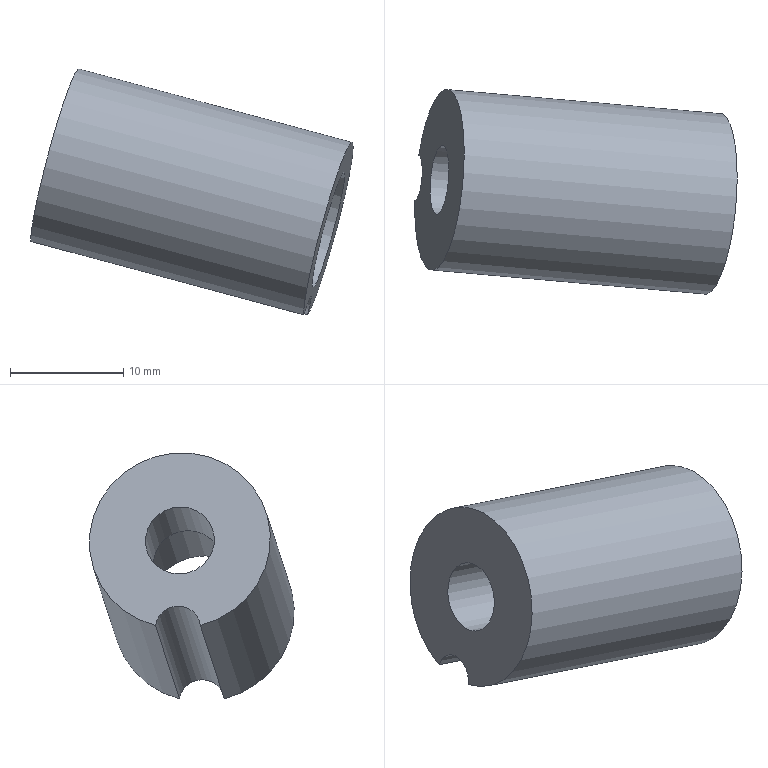Part | NX | features solid 2 | 1 solid | 7 faces | box 28.411 x 18.048 x 21.684 mm | volume 3144 mm3 | cylinder 4 | plane 3 | commonest cylinder face diameters 4 x1 6.1 x1 10.6 x1 16 x1
STEP:
#1=CARTESIAN_POINT('',(-364.408,301.962,-18.156));
#2=VERTEX_POINT('',#1);
#3=CARTESIAN_POINT('',(-388.464,304.067,-11.685));
#4=VERTEX_POINT('',#3);
#5=CARTESIAN_POINT('',(-376.436,303.015,-14.921));
#6=DIRECTION('',(-0.9623,0.08419,0.2588));
#7=VECTOR('',#6,1000.);
#8=LINE('',#5,#7);
#9=EDGE_CURVE('',#2,#4,#8,.T.);
#10=ORIENTED_EDGE('',*,*,#9,.T.);
#11=CARTESIAN_POINT('',(-388.81,300.113,-11.685));
#12=VERTEX_POINT('',#11);
#13=CARTESIAN_POINT('',(-386.639,301.915,-4.199));
#14=DIRECTION('',(0.9623,-0.08419,-0.2588));
#15=DIRECTION('',(-0.2578,0.02256,-0.9659));
#16=AXIS2_PLACEMENT_3D('',#13,#14,#15);
#17=CIRCLE('',#16,8.);
#18=EDGE_CURVE('',#4,#12,#17,.T.);
#19=ORIENTED_EDGE('',*,*,#18,.T.);
#20=CARTESIAN_POINT('',(-364.754,298.009,-18.156));
#21=VERTEX_POINT('',#20);
#22=CARTESIAN_POINT('',(-376.782,299.061,-14.921));
#23=DIRECTION('',(-0.9623,0.08419,0.2588));
#24=VECTOR('',#23,1000.);
#25=LINE('',#22,#24);
#26=EDGE_CURVE('',#12,#21,#25,.F.);
#27=ORIENTED_EDGE('',*,*,#26,.T.);
#28=CARTESIAN_POINT('',(-362.583,299.811,-10.67));
#29=DIRECTION('',(0.9623,-0.08419,-0.2588));
#30=DIRECTION('',(-0.2578,0.02256,-0.9659));
#31=AXIS2_PLACEMENT_3D('',#28,#29,#30);
#32=CIRCLE('',#31,8.);
#33=EDGE_CURVE('',#2,#21,#32,.T.);
#34=ORIENTED_EDGE('',*,*,#33,.F.);
#35=EDGE_LOOP('',(#10,#19,#27,#34));
#36=FACE_BOUND('',#35,.T.);
#37=CARTESIAN_POINT('',(-362.583,299.811,-10.67));
#38=DIRECTION('',(-0.9623,0.08419,0.2588));
#39=DIRECTION('',(-0.2578,0.02256,-0.9659));
#40=AXIS2_PLACEMENT_3D('',#37,#38,#39);
#41=CYLINDRICAL_SURFACE('',#40,8.);
#42=ADVANCED_FACE('',(#36),#41,.T.);
#43=CARTESIAN_POINT('',(-363.949,299.93,-15.789));
#44=VERTEX_POINT('',#43);
#45=CARTESIAN_POINT('',(-362.583,299.811,-10.67));
#46=DIRECTION('',(0.9623,-0.08419,-0.2588));
#47=DIRECTION('',(-0.2578,0.02256,-0.9659));
#48=AXIS2_PLACEMENT_3D('',#45,#46,#47);
#49=CIRCLE('',#48,5.3);
#50=EDGE_CURVE('',#44,#44,#49,.T.);
#51=ORIENTED_EDGE('',*,*,#50,.F.);
#52=EDGE_LOOP('',(#51));
#53=FACE_BOUND('',#52,.T.);
#54=ORIENTED_EDGE('',*,*,#33,.T.);
#55=CARTESIAN_POINT('',(-364.645,299.991,-18.397));
#56=DIRECTION('',(0.9623,-0.08419,-0.2588));
#57=DIRECTION('',(-0.2578,0.02256,-0.9659));
#58=AXIS2_PLACEMENT_3D('',#55,#56,#57);
#59=CIRCLE('',#58,2.);
#60=EDGE_CURVE('',#2,#21,#59,.T.);
#61=ORIENTED_EDGE('',*,*,#60,.F.);
#62=EDGE_LOOP('',(#54,#61));
#63=FACE_BOUND('',#62,.T.);
#64=CARTESIAN_POINT('',(-362.583,299.811,-10.67));
#65=DIRECTION('',(-0.9623,0.08419,0.2588));
#66=DIRECTION('',(-0.2578,0.02256,-0.9659));
#67=AXIS2_PLACEMENT_3D('',#64,#65,#66);
#68=PLANE('',#67);
#69=ADVANCED_FACE('',(#53,#63),#68,.F.);
#70=CARTESIAN_POINT('',(-387.425,301.984,-7.146));
#71=VERTEX_POINT('',#70);
#72=CARTESIAN_POINT('',(-386.639,301.915,-4.199));
#73=DIRECTION('',(0.9623,-0.08419,-0.2588));
#74=DIRECTION('',(-0.2578,0.02256,-0.9659));
#75=AXIS2_PLACEMENT_3D('',#72,#73,#74);
#76=CIRCLE('',#75,3.05);
#77=EDGE_CURVE('',#71,#71,#76,.T.);
#78=ORIENTED_EDGE('',*,*,#77,.T.);
#79=EDGE_LOOP('',(#78));
#80=FACE_BOUND('',#79,.T.);
#81=CARTESIAN_POINT('',(-388.701,302.096,-11.927));
#82=DIRECTION('',(0.9623,-0.08419,-0.2588));
#83=DIRECTION('',(-0.2578,0.02256,-0.9659));
#84=AXIS2_PLACEMENT_3D('',#81,#82,#83);
#85=CIRCLE('',#84,2.);
#86=EDGE_CURVE('',#4,#12,#85,.T.);
#87=ORIENTED_EDGE('',*,*,#86,.T.);
#88=ORIENTED_EDGE('',*,*,#18,.F.);
#89=EDGE_LOOP('',(#87,#88));
#90=FACE_BOUND('',#89,.T.);
#91=CARTESIAN_POINT('',(-386.639,301.915,-4.199));
#92=DIRECTION('',(-0.9623,0.08419,0.2588));
#93=DIRECTION('',(-0.2578,0.02256,-0.9659));
#94=AXIS2_PLACEMENT_3D('',#91,#92,#93);
#95=PLANE('',#94);
#96=ADVANCED_FACE('',(#80,#90),#95,.T.);
#97=ORIENTED_EDGE('',*,*,#50,.T.);
#98=EDGE_LOOP('',(#97));
#99=FACE_BOUND('',#98,.T.);
#100=CARTESIAN_POINT('',(-380.307,301.361,-11.389));
#101=VERTEX_POINT('',#100);
#102=CARTESIAN_POINT('',(-378.941,301.242,-6.27));
#103=DIRECTION('',(0.9623,-0.08419,-0.2588));
#104=DIRECTION('',(-0.2578,0.02256,-0.9659));
#105=AXIS2_PLACEMENT_3D('',#102,#103,#104);
#106=CIRCLE('',#105,5.3);
#107=EDGE_CURVE('',#101,#101,#106,.T.);
#108=ORIENTED_EDGE('',*,*,#107,.F.);
#109=EDGE_LOOP('',(#108));
#110=FACE_BOUND('',#109,.T.);
#111=CARTESIAN_POINT('',(-362.583,299.811,-10.67));
#112=DIRECTION('',(-0.9623,0.08419,0.2588));
#113=DIRECTION('',(-0.2578,0.02256,-0.9659));
#114=AXIS2_PLACEMENT_3D('',#111,#112,#113);
#115=CYLINDRICAL_SURFACE('',#114,5.3);
#116=ADVANCED_FACE('',(#99,#110),#115,.F.);
#117=CARTESIAN_POINT('',(-379.727,301.311,-9.216));
#118=VERTEX_POINT('',#117);
#119=CARTESIAN_POINT('',(-378.941,301.242,-6.27));
#120=DIRECTION('',(0.9623,-0.08419,-0.2588));
#121=DIRECTION('',(-0.2578,0.02256,-0.9659));
#122=AXIS2_PLACEMENT_3D('',#119,#120,#121);
#123=CIRCLE('',#122,3.05);
#124=EDGE_CURVE('',#118,#118,#123,.T.);
#125=ORIENTED_EDGE('',*,*,#124,.F.);
#126=EDGE_LOOP('',(#125));
#127=FACE_BOUND('',#126,.T.);
#128=ORIENTED_EDGE('',*,*,#107,.T.);
#129=EDGE_LOOP('',(#128));
#130=FACE_BOUND('',#129,.T.);
#131=CARTESIAN_POINT('',(-378.941,301.242,-6.27));
#132=DIRECTION('',(-0.9623,0.08419,0.2588));
#133=DIRECTION('',(-0.2578,0.02256,-0.9659));
#134=AXIS2_PLACEMENT_3D('',#131,#132,#133);
#135=PLANE('',#134);
#136=ADVANCED_FACE('',(#127,#130),#135,.F.);
#137=ORIENTED_EDGE('',*,*,#9,.F.);
#138=ORIENTED_EDGE('',*,*,#60,.T.);
#139=ORIENTED_EDGE('',*,*,#26,.F.);
#140=ORIENTED_EDGE('',*,*,#86,.F.);
#141=EDGE_LOOP('',(#137,#138,#139,#140));
#142=FACE_BOUND('',#141,.T.);
#143=CARTESIAN_POINT('',(-364.645,299.991,-18.397));
#144=DIRECTION('',(-0.9623,0.08419,0.2588));
#145=DIRECTION('',(-0.2578,0.02256,-0.9659));
#146=AXIS2_PLACEMENT_3D('',#143,#144,#145);
#147=CYLINDRICAL_SURFACE('',#146,2.);
#148=ADVANCED_FACE('',(#142),#147,.F.);
#149=ORIENTED_EDGE('',*,*,#77,.F.);
#150=EDGE_LOOP('',(#149));
#151=FACE_BOUND('',#150,.T.);
#152=ORIENTED_EDGE('',*,*,#124,.T.);
#153=EDGE_LOOP('',(#152));
#154=FACE_BOUND('',#153,.T.);
#155=CARTESIAN_POINT('',(-362.583,299.811,-10.67));
#156=DIRECTION('',(-0.9623,0.08419,0.2588));
#157=DIRECTION('',(-0.2578,0.02256,-0.9659));
#158=AXIS2_PLACEMENT_3D('',#155,#156,#157);
#159=CYLINDRICAL_SURFACE('',#158,3.05);
#160=ADVANCED_FACE('',(#151,#154),#159,.F.);
#161=CLOSED_SHELL('',(#42,#69,#96,#116,#136,#148,#160));
#162=MANIFOLD_SOLID_BREP('',#161);
#163=(LENGTH_UNIT()NAMED_UNIT(*)SI_UNIT(.MILLI.,.METRE.));
#164=UNCERTAINTY_MEASURE_WITH_UNIT(LENGTH_MEASURE(0.00001),#163,'','');
#165=(NAMED_UNIT(*)PLANE_ANGLE_UNIT()SI_UNIT($,.RADIAN.));
#166=(NAMED_UNIT(*)SI_UNIT($,.STERADIAN.)SOLID_ANGLE_UNIT());
#167=(GEOMETRIC_REPRESENTATION_CONTEXT(3)GLOBAL_UNCERTAINTY_ASSIGNED_CONTEXT((#164))GLOBAL_UNIT_ASSIGNED_CONTEXT((#163,#165,#166))REPRESENTATION_CONTEXT('',''));
#168=ADVANCED_BREP_SHAPE_REPRESENTATION('',(#162),#167);